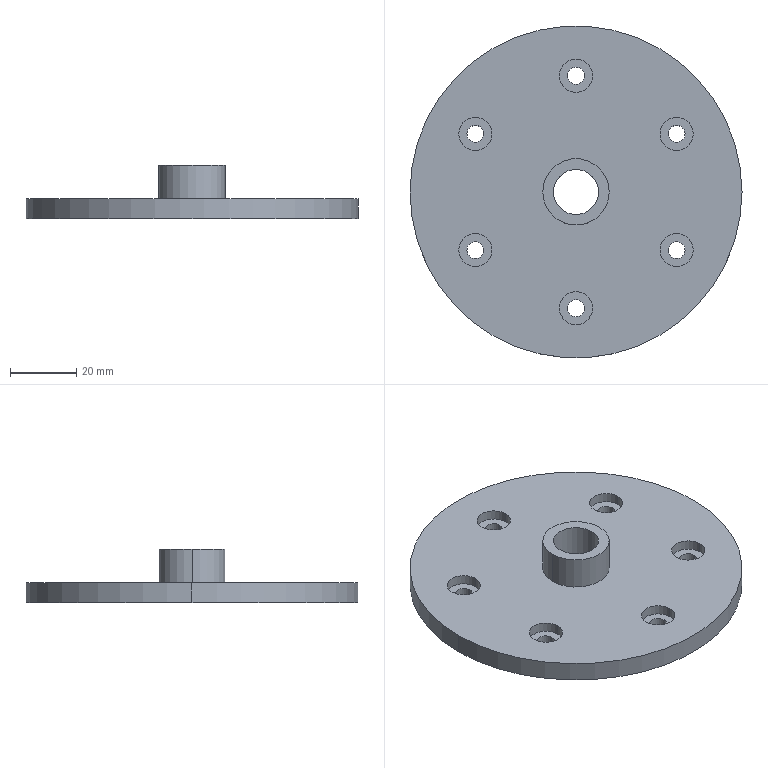CAM job | NX | 3-axis milling, drilling | part box 100 x 100 x 16 mm | stock box 106 x 106 x 22 mm
Tools:
number,name,description,diameter,corner_radius,flute_length,length,flutes
1,D14开粗,,14.0,0.0,50.0,75.0,2
3,D6点钻,,6.0,0.0,15.0,30.0,1
4,D5.1钻头,,5.1,0.0,35.0,50.0,2
5,D10开粗,,10.0,0.0,50.0,75.0,2
2,D16精光,,16.0,0.0,50.0,75.0,2
6,3-8丝锥,,14.9,0.0,35.0,50.0,4
Operations:
program,operation,operation_type,tool,method,geometry_group,spindle_rpm,surface_speed,feed_per_tooth,feed_cut,feed_plunge,cut_length_mm,path_length_mm,cut_time_min,machine_time_min
G54,ADAPTIVE_MILLING,CavityMilling,D14开粗,METHOD,WORKPIECE,4500.0,100.0,0.1178,3000.0,100.0,8808.505,8936.52,2.936,2.949
G54,PLANAR_MILL,PlanarMilling,D14开粗,METHOD,WORKPIECE,4500.0,197.0,0.1111,1000.0,100.0,70.442,106.442,0.0704,0.074
G54,DRILLING,Operation,D6点钻,METHOD,WORKPIECE,2000.0,37.0,0.1,200.0,0.0,27.0,304.642,0.135,0.1628
G54,DRILLING_COPY,Operation,D5.1钻头,METHOD,WORKPIECE,2000.0,37.0,0.1,200.0,0.0,72.0,394.642,0.36,0.3923
G54,DRILLING_COPY_COPY,Operation,D10开粗,METHOD,WORKPIECE,1600.0,50.0,0.0312,100.0,0.0,36.0,322.642,0.36,0.3887
G54,HOLE_MILLING,CylinderMilling,D10开粗,METHOD,WORKPIECE,3500.0,109.0,0.0857,600.0,100.0,488.866,547.866,0.8148,0.8207
G54,PLANAR_MILL_1,PlanarMilling,D16精光,METHOD,WORKPIECE,3500.0,175.0,0.1143,800.0,100.0,1070.351,1124.351,1.338,1.343
G54,PLANAR_MILL_1_COPY,PlanarMilling,D16精光,METHOD,WORKPIECE,3500.0,175.0,0.1143,800.0,100.0,128.522,184.502,0.1607,0.1663
G54,PLANAR_MILL_1_COPY_COPY,PlanarMilling,D16精光,METHOD,WORKPIECE,3500.0,175.0,0.1143,800.0,100.0,761.352,831.332,0.9517,0.9587
G54,PLANAR_MILL_2,PlanarMilling,D6点钻,METHOD,WORKPIECE,3000.0,56.0,0.3333,1000.0,100.0,86.681,126.681,0.0867,0.0907
G54,PLANAR_MILL_2_COPY,PlanarMilling,D6点钻,METHOD,WORKPIECE,3000.0,56.0,0.3333,1000.0,100.0,41.056,81.056,0.0411,0.0451
G54,PLANAR_MILL_3,PlanarMilling,D6点钻,METHOD,WORKPIECE,3000.0,56.0,0.3333,1000.0,100.0,155.947,689.118,0.1559,0.2093
G54,PLANAR_MILL_3_COPY,PlanarMilling,D6点钻,METHOD,WORKPIECE,3000.0,56.0,0.3333,1000.0,100.0,333.867,393.867,0.3339,0.3399
G54,DRILLING_COPY_1,Operation,D6点钻,METHOD,WORKPIECE,3000.0,56.0,0.0667,200.0,0.0,27.6,322.977,0.138,0.1675
G54,DRILLING_1,Operation,3-8丝锥,METHOD,WORKPIECE,200.0,9.0,0.0029,2.309,0.0,23.0,86.0,9.961,9.967
G55,ADAPTIVE_MILLING_1,CavityMilling,D14开粗,METHOD,WORKPIECE_1,4500.0,197.0,0.3333,3000.0,100.0,8878.166,8911.866,2.959,2.963
G55,FLOOR_WALL,VolumeBased25DMillingOperation,D16精光,METHOD,WORKPIECE_1,3500.0,175.0,0.1429,1000.0,100.0,789.51,823.51,0.7895,0.7929
G55,PLANAR_MILL_4,PlanarMilling,D6点钻,METHOD,WORKPIECE_1,3500.0,175.0,0.1429,1000.0,100.0,337.009,377.009,0.337,0.341